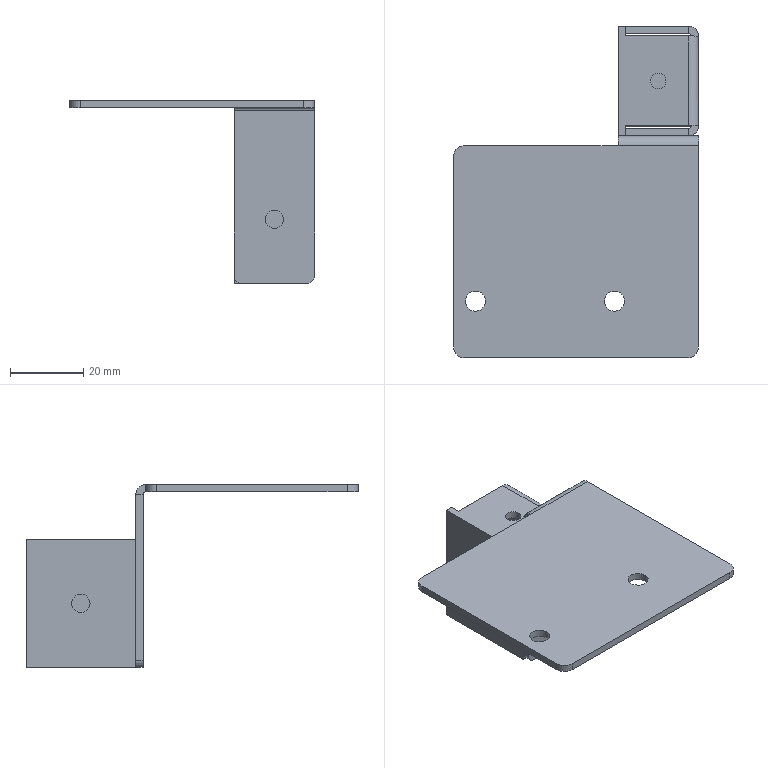Part | SolidWorks | features ICE 5, EdgeFlange 2, Fillet 2, FlatPattern 2, HoleWzd 2, SMBaseFlange 2, SheetMetal 2, MirrorSolid 1 | 2 solids | 68 faces | box 67 x 90.75 x 50 mm | volume 17594 mm3 | plane 33 | cylinder 27 | spline 8 | commonest cylinder face diameters 5.5 x9 5 x6 1.5 x5 6 x3 4 x2 4.2 x2